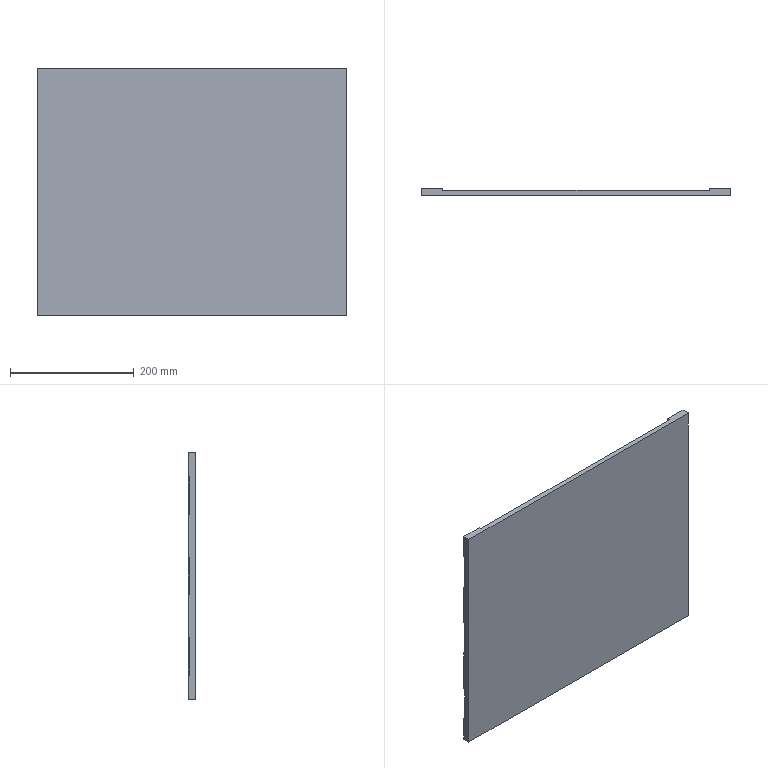Part | SolidWorks | features ICE 4, Extrusion 1, Fillet 1 | 1 solid | 28 faces | box 500 x 11.75 x 400 mm | volume 1696904 mm3 | plane 22 | cylinder 6 | commonest cylinder face diameters 10 x6
STEP:
#1=CARTESIAN_POINT('',(0.,9.75,-360.));
#2=VERTEX_POINT('',#1);
#3=CARTESIAN_POINT('',(0.,11.75,-360.));
#4=VERTEX_POINT('',#3);
#5=CARTESIAN_POINT('',(0.,9.75,-360.));
#6=DIRECTION('',(0.,1.,0.));
#7=VECTOR('',#6,1000.);
#8=LINE('',#5,#7);
#9=EDGE_CURVE('',#2,#4,#8,.T.);
#10=ORIENTED_EDGE('',*,*,#9,.T.);
#11=CARTESIAN_POINT('',(0.,11.75,-400.));
#12=VERTEX_POINT('',#11);
#13=CARTESIAN_POINT('',(0.,11.75,-400.));
#14=DIRECTION('',(0.,0.,1.));
#15=VECTOR('',#14,1000.);
#16=LINE('',#13,#15);
#17=EDGE_CURVE('',#12,#4,#16,.T.);
#18=ORIENTED_EDGE('',*,*,#17,.F.);
#19=CARTESIAN_POINT('',(0.,0.,-400.));
#20=VERTEX_POINT('',#19);
#21=CARTESIAN_POINT('',(0.,0.,-400.));
#22=DIRECTION('',(0.,-1.,0.));
#23=VECTOR('',#22,1000.);
#24=LINE('',#21,#23);
#25=EDGE_CURVE('',#12,#20,#24,.T.);
#26=ORIENTED_EDGE('',*,*,#25,.T.);
#27=CARTESIAN_POINT('',(0.,0.,0.));
#28=VERTEX_POINT('',#27);
#29=CARTESIAN_POINT('',(0.,0.,-400.));
#30=DIRECTION('',(0.,0.,1.));
#31=VECTOR('',#30,1000.);
#32=LINE('',#29,#31);
#33=EDGE_CURVE('',#20,#28,#32,.T.);
#34=ORIENTED_EDGE('',*,*,#33,.T.);
#35=CARTESIAN_POINT('',(0.,11.75,0.));
#36=VERTEX_POINT('',#35);
#37=CARTESIAN_POINT('',(0.,0.,0.));
#38=DIRECTION('',(0.,-1.,0.));
#39=VECTOR('',#38,1000.);
#40=LINE('',#37,#39);
#41=EDGE_CURVE('',#36,#28,#40,.T.);
#42=ORIENTED_EDGE('',*,*,#41,.F.);
#43=CARTESIAN_POINT('',(0.,11.75,-40.));
#44=VERTEX_POINT('',#43);
#45=CARTESIAN_POINT('',(0.,11.75,-400.));
#46=DIRECTION('',(0.,0.,1.));
#47=VECTOR('',#46,1000.);
#48=LINE('',#45,#47);
#49=EDGE_CURVE('',#44,#36,#48,.T.);
#50=ORIENTED_EDGE('',*,*,#49,.F.);
#51=CARTESIAN_POINT('',(0.,9.75,-40.));
#52=VERTEX_POINT('',#51);
#53=CARTESIAN_POINT('',(0.,9.75,-40.));
#54=DIRECTION('',(0.,1.,0.));
#55=VECTOR('',#54,1000.);
#56=LINE('',#53,#55);
#57=EDGE_CURVE('',#52,#44,#56,.T.);
#58=ORIENTED_EDGE('',*,*,#57,.F.);
#59=CARTESIAN_POINT('',(0.,9.75,-100.));
#60=VERTEX_POINT('',#59);
#61=CARTESIAN_POINT('',(0.,9.75,-40.));
#62=DIRECTION('',(0.,0.,1.));
#63=VECTOR('',#62,1000.);
#64=LINE('',#61,#63);
#65=EDGE_CURVE('',#60,#52,#64,.T.);
#66=ORIENTED_EDGE('',*,*,#65,.F.);
#67=CARTESIAN_POINT('',(0.,11.75,-100.));
#68=VERTEX_POINT('',#67);
#69=CARTESIAN_POINT('',(0.,9.75,-100.));
#70=DIRECTION('',(0.,1.,0.));
#71=VECTOR('',#70,1000.);
#72=LINE('',#69,#71);
#73=EDGE_CURVE('',#60,#68,#72,.T.);
#74=ORIENTED_EDGE('',*,*,#73,.T.);
#75=CARTESIAN_POINT('',(0.,11.75,-170.));
#76=VERTEX_POINT('',#75);
#77=CARTESIAN_POINT('',(0.,11.75,-400.));
#78=DIRECTION('',(0.,0.,1.));
#79=VECTOR('',#78,1000.);
#80=LINE('',#77,#79);
#81=EDGE_CURVE('',#76,#68,#80,.T.);
#82=ORIENTED_EDGE('',*,*,#81,.F.);
#83=CARTESIAN_POINT('',(0.,9.75,-170.));
#84=VERTEX_POINT('',#83);
#85=CARTESIAN_POINT('',(0.,9.75,-170.));
#86=DIRECTION('',(0.,1.,0.));
#87=VECTOR('',#86,1000.);
#88=LINE('',#85,#87);
#89=EDGE_CURVE('',#84,#76,#88,.T.);
#90=ORIENTED_EDGE('',*,*,#89,.F.);
#91=CARTESIAN_POINT('',(0.,9.75,-230.));
#92=VERTEX_POINT('',#91);
#93=CARTESIAN_POINT('',(0.,9.75,-230.));
#94=DIRECTION('',(0.,0.,1.));
#95=VECTOR('',#94,1000.);
#96=LINE('',#93,#95);
#97=EDGE_CURVE('',#92,#84,#96,.T.);
#98=ORIENTED_EDGE('',*,*,#97,.F.);
#99=CARTESIAN_POINT('',(0.,11.75,-230.));
#100=VERTEX_POINT('',#99);
#101=CARTESIAN_POINT('',(0.,9.75,-230.));
#102=DIRECTION('',(0.,1.,0.));
#103=VECTOR('',#102,1000.);
#104=LINE('',#101,#103);
#105=EDGE_CURVE('',#92,#100,#104,.T.);
#106=ORIENTED_EDGE('',*,*,#105,.T.);
#107=CARTESIAN_POINT('',(0.,11.75,-300.));
#108=VERTEX_POINT('',#107);
#109=CARTESIAN_POINT('',(0.,11.75,-400.));
#110=DIRECTION('',(0.,0.,1.));
#111=VECTOR('',#110,1000.);
#112=LINE('',#109,#111);
#113=EDGE_CURVE('',#108,#100,#112,.T.);
#114=ORIENTED_EDGE('',*,*,#113,.F.);
#115=CARTESIAN_POINT('',(0.,9.75,-300.));
#116=VERTEX_POINT('',#115);
#117=CARTESIAN_POINT('',(0.,9.75,-300.));
#118=DIRECTION('',(0.,1.,0.));
#119=VECTOR('',#118,1000.);
#120=LINE('',#117,#119);
#121=EDGE_CURVE('',#116,#108,#120,.T.);
#122=ORIENTED_EDGE('',*,*,#121,.F.);
#123=CARTESIAN_POINT('',(0.,9.75,-360.));
#124=DIRECTION('',(0.,0.,1.));
#125=VECTOR('',#124,1000.);
#126=LINE('',#123,#125);
#127=EDGE_CURVE('',#2,#116,#126,.T.);
#128=ORIENTED_EDGE('',*,*,#127,.F.);
#129=EDGE_LOOP('',(#10,#18,#26,#34,#42,#50,#58,#66,#74,#82,#90,#98,#106,#114,#122,#128));
#130=FACE_OUTER_BOUND('',#129,.T.);
#131=CARTESIAN_POINT('',(0.,0.,-400.));
#132=DIRECTION('',(-1.,0.,0.));
#133=DIRECTION('',(0.,0.,1.));
#134=AXIS2_PLACEMENT_3D('',#131,#132,#133);
#135=PLANE('',#134);
#136=ADVANCED_FACE('',(#130),#135,.T.);
#137=CARTESIAN_POINT('',(500.,11.75,0.));
#138=VERTEX_POINT('',#137);
#139=CARTESIAN_POINT('',(500.,11.75,-400.));
#140=VERTEX_POINT('',#139);
#141=CARTESIAN_POINT('',(500.,11.75,-400.));
#142=DIRECTION('',(0.,0.,-1.));
#143=VECTOR('',#142,1000.);
#144=LINE('',#141,#143);
#145=EDGE_CURVE('',#138,#140,#144,.T.);
#146=ORIENTED_EDGE('',*,*,#145,.F.);
#147=CARTESIAN_POINT('',(500.,0.,0.));
#148=VERTEX_POINT('',#147);
#149=CARTESIAN_POINT('',(500.,0.,0.));
#150=DIRECTION('',(0.,1.,0.));
#151=VECTOR('',#150,1000.);
#152=LINE('',#149,#151);
#153=EDGE_CURVE('',#148,#138,#152,.T.);
#154=ORIENTED_EDGE('',*,*,#153,.F.);
#155=CARTESIAN_POINT('',(500.,0.,-400.));
#156=VERTEX_POINT('',#155);
#157=CARTESIAN_POINT('',(500.,0.,-400.));
#158=DIRECTION('',(0.,0.,1.));
#159=VECTOR('',#158,1000.);
#160=LINE('',#157,#159);
#161=EDGE_CURVE('',#156,#148,#160,.T.);
#162=ORIENTED_EDGE('',*,*,#161,.F.);
#163=CARTESIAN_POINT('',(500.,0.,-400.));
#164=DIRECTION('',(0.,1.,0.));
#165=VECTOR('',#164,1000.);
#166=LINE('',#163,#165);
#167=EDGE_CURVE('',#156,#140,#166,.T.);
#168=ORIENTED_EDGE('',*,*,#167,.T.);
#169=EDGE_LOOP('',(#146,#154,#162,#168));
#170=FACE_OUTER_BOUND('',#169,.T.);
#171=CARTESIAN_POINT('',(500.,0.,-400.));
#172=DIRECTION('',(1.,0.,0.));
#173=DIRECTION('',(0.,0.,-1.));
#174=AXIS2_PLACEMENT_3D('',#171,#172,#173);
#175=PLANE('',#174);
#176=ADVANCED_FACE('',(#170),#175,.T.);
#177=CARTESIAN_POINT('',(465.,11.75,-400.));
#178=VERTEX_POINT('',#177);
#179=CARTESIAN_POINT('',(-22.479,11.75,-400.));
#180=DIRECTION('',(1.,0.,0.));
#181=VECTOR('',#180,1000.);
#182=LINE('',#179,#181);
#183=EDGE_CURVE('',#178,#140,#182,.T.);
#184=ORIENTED_EDGE('',*,*,#183,.T.);
#185=ORIENTED_EDGE('',*,*,#167,.F.);
#186=CARTESIAN_POINT('',(0.,0.,-400.));
#187=DIRECTION('',(1.,0.,0.));
#188=VECTOR('',#187,1000.);
#189=LINE('',#186,#188);
#190=EDGE_CURVE('',#20,#156,#189,.T.);
#191=ORIENTED_EDGE('',*,*,#190,.F.);
#192=ORIENTED_EDGE('',*,*,#25,.F.);
#193=CARTESIAN_POINT('',(35.,11.75,-400.));
#194=VERTEX_POINT('',#193);
#195=CARTESIAN_POINT('',(-22.479,11.75,-400.));
#196=DIRECTION('',(1.,0.,0.));
#197=VECTOR('',#196,1000.);
#198=LINE('',#195,#197);
#199=EDGE_CURVE('',#12,#194,#198,.T.);
#200=ORIENTED_EDGE('',*,*,#199,.T.);
#201=CARTESIAN_POINT('',(35.,8.,-400.));
#202=VERTEX_POINT('',#201);
#203=CARTESIAN_POINT('',(35.,16.,-400.));
#204=DIRECTION('',(0.,-1.,0.));
#205=VECTOR('',#204,1000.);
#206=LINE('',#203,#205);
#207=EDGE_CURVE('',#194,#202,#206,.T.);
#208=ORIENTED_EDGE('',*,*,#207,.T.);
#209=CARTESIAN_POINT('',(465.,8.,-400.));
#210=VERTEX_POINT('',#209);
#211=CARTESIAN_POINT('',(35.,8.,-400.));
#212=DIRECTION('',(1.,0.,0.));
#213=VECTOR('',#212,1000.);
#214=LINE('',#211,#213);
#215=EDGE_CURVE('',#202,#210,#214,.T.);
#216=ORIENTED_EDGE('',*,*,#215,.T.);
#217=CARTESIAN_POINT('',(465.,16.,-400.));
#218=DIRECTION('',(0.,1.,0.));
#219=VECTOR('',#218,1000.);
#220=LINE('',#217,#219);
#221=EDGE_CURVE('',#210,#178,#220,.T.);
#222=ORIENTED_EDGE('',*,*,#221,.T.);
#223=EDGE_LOOP('',(#184,#185,#191,#192,#200,#208,#216,#222));
#224=FACE_OUTER_BOUND('',#223,.T.);
#225=CARTESIAN_POINT('',(0.,0.,-400.));
#226=DIRECTION('',(0.,0.,-1.));
#227=DIRECTION('',(-1.,0.,0.));
#228=AXIS2_PLACEMENT_3D('',#225,#226,#227);
#229=PLANE('',#228);
#230=ADVANCED_FACE('',(#224),#229,.T.);
#231=ORIENTED_EDGE('',*,*,#153,.T.);
#232=CARTESIAN_POINT('',(465.,11.75,0.));
#233=VERTEX_POINT('',#232);
#234=CARTESIAN_POINT('',(-22.479,11.75,0.));
#235=DIRECTION('',(1.,0.,0.));
#236=VECTOR('',#235,1000.);
#237=LINE('',#234,#236);
#238=EDGE_CURVE('',#233,#138,#237,.T.);
#239=ORIENTED_EDGE('',*,*,#238,.F.);
#240=CARTESIAN_POINT('',(465.,8.,0.));
#241=VERTEX_POINT('',#240);
#242=CARTESIAN_POINT('',(465.,16.,0.));
#243=DIRECTION('',(0.,1.,0.));
#244=VECTOR('',#243,1000.);
#245=LINE('',#242,#244);
#246=EDGE_CURVE('',#241,#233,#245,.T.);
#247=ORIENTED_EDGE('',*,*,#246,.F.);
#248=CARTESIAN_POINT('',(35.,8.,0.));
#249=VERTEX_POINT('',#248);
#250=CARTESIAN_POINT('',(35.,8.,0.));
#251=DIRECTION('',(1.,0.,0.));
#252=VECTOR('',#251,1000.);
#253=LINE('',#250,#252);
#254=EDGE_CURVE('',#249,#241,#253,.T.);
#255=ORIENTED_EDGE('',*,*,#254,.F.);
#256=CARTESIAN_POINT('',(35.,11.75,0.));
#257=VERTEX_POINT('',#256);
#258=CARTESIAN_POINT('',(35.,16.,0.));
#259=DIRECTION('',(0.,-1.,0.));
#260=VECTOR('',#259,1000.);
#261=LINE('',#258,#260);
#262=EDGE_CURVE('',#257,#249,#261,.T.);
#263=ORIENTED_EDGE('',*,*,#262,.F.);
#264=CARTESIAN_POINT('',(-22.479,11.75,0.));
#265=DIRECTION('',(1.,0.,0.));
#266=VECTOR('',#265,1000.);
#267=LINE('',#264,#266);
#268=EDGE_CURVE('',#36,#257,#267,.T.);
#269=ORIENTED_EDGE('',*,*,#268,.F.);
#270=ORIENTED_EDGE('',*,*,#41,.T.);
#271=CARTESIAN_POINT('',(0.,0.,0.));
#272=DIRECTION('',(1.,0.,0.));
#273=VECTOR('',#272,1000.);
#274=LINE('',#271,#273);
#275=EDGE_CURVE('',#28,#148,#274,.T.);
#276=ORIENTED_EDGE('',*,*,#275,.T.);
#277=EDGE_LOOP('',(#231,#239,#247,#255,#263,#269,#270,#276));
#278=FACE_OUTER_BOUND('',#277,.T.);
#279=CARTESIAN_POINT('',(0.,0.,0.));
#280=DIRECTION('',(0.,0.,-1.));
#281=DIRECTION('',(-1.,0.,0.));
#282=AXIS2_PLACEMENT_3D('',#279,#280,#281);
#283=PLANE('',#282);
#284=ADVANCED_FACE('',(#278),#283,.F.);
#285=ORIENTED_EDGE('',*,*,#207,.F.);
#286=CARTESIAN_POINT('',(35.,11.75,-400.));
#287=DIRECTION('',(0.,0.,1.));
#288=VECTOR('',#287,1000.);
#289=LINE('',#286,#288);
#290=EDGE_CURVE('',#194,#257,#289,.T.);
#291=ORIENTED_EDGE('',*,*,#290,.T.);
#292=ORIENTED_EDGE('',*,*,#262,.T.);
#293=CARTESIAN_POINT('',(35.,8.,-400.));
#294=DIRECTION('',(0.,0.,1.));
#295=VECTOR('',#294,1000.);
#296=LINE('',#293,#295);
#297=EDGE_CURVE('',#202,#249,#296,.T.);
#298=ORIENTED_EDGE('',*,*,#297,.F.);
#299=EDGE_LOOP('',(#285,#291,#292,#298));
#300=FACE_OUTER_BOUND('',#299,.T.);
#301=CARTESIAN_POINT('',(35.,16.,-400.));
#302=DIRECTION('',(-1.,0.,0.));
#303=DIRECTION('',(0.,0.,1.));
#304=AXIS2_PLACEMENT_3D('',#301,#302,#303);
#305=PLANE('',#304);
#306=ADVANCED_FACE('',(#300),#305,.F.);
#307=ORIENTED_EDGE('',*,*,#246,.T.);
#308=CARTESIAN_POINT('',(465.,11.75,-400.));
#309=DIRECTION('',(0.,0.,-1.));
#310=VECTOR('',#309,1000.);
#311=LINE('',#308,#310);
#312=EDGE_CURVE('',#233,#178,#311,.T.);
#313=ORIENTED_EDGE('',*,*,#312,.T.);
#314=ORIENTED_EDGE('',*,*,#221,.F.);
#315=CARTESIAN_POINT('',(465.,8.,-400.));
#316=DIRECTION('',(0.,0.,1.));
#317=VECTOR('',#316,1000.);
#318=LINE('',#315,#317);
#319=EDGE_CURVE('',#210,#241,#318,.T.);
#320=ORIENTED_EDGE('',*,*,#319,.T.);
#321=EDGE_LOOP('',(#307,#313,#314,#320));
#322=FACE_OUTER_BOUND('',#321,.T.);
#323=CARTESIAN_POINT('',(465.,16.,-400.));
#324=DIRECTION('',(1.,0.,0.));
#325=DIRECTION('',(0.,0.,-1.));
#326=AXIS2_PLACEMENT_3D('',#323,#324,#325);
#327=PLANE('',#326);
#328=ADVANCED_FACE('',(#322),#327,.F.);
#329=ORIENTED_EDGE('',*,*,#275,.F.);
#330=ORIENTED_EDGE('',*,*,#33,.F.);
#331=ORIENTED_EDGE('',*,*,#190,.T.);
#332=ORIENTED_EDGE('',*,*,#161,.T.);
#333=EDGE_LOOP('',(#329,#330,#331,#332));
#334=FACE_OUTER_BOUND('',#333,.T.);
#335=CARTESIAN_POINT('',(0.,0.,-400.));
#336=DIRECTION('',(0.,-1.,0.));
#337=DIRECTION('',(0.,0.,-1.));
#338=AXIS2_PLACEMENT_3D('',#335,#336,#337);
#339=PLANE('',#338);
#340=ADVANCED_FACE('',(#334),#339,.T.);
#341=ORIENTED_EDGE('',*,*,#254,.T.);
#342=ORIENTED_EDGE('',*,*,#319,.F.);
#343=ORIENTED_EDGE('',*,*,#215,.F.);
#344=ORIENTED_EDGE('',*,*,#297,.T.);
#345=EDGE_LOOP('',(#341,#342,#343,#344));
#346=FACE_OUTER_BOUND('',#345,.T.);
#347=CARTESIAN_POINT('',(35.,8.,-400.));
#348=DIRECTION('',(0.,-1.,0.));
#349=DIRECTION('',(1.,0.,0.));
#350=AXIS2_PLACEMENT_3D('',#347,#348,#349);
#351=PLANE('',#350);
#352=ADVANCED_FACE('',(#346),#351,.F.);
#353=ORIENTED_EDGE('',*,*,#145,.T.);
#354=ORIENTED_EDGE('',*,*,#183,.F.);
#355=ORIENTED_EDGE('',*,*,#312,.F.);
#356=ORIENTED_EDGE('',*,*,#238,.T.);
#357=EDGE_LOOP('',(#353,#354,#355,#356));
#358=FACE_OUTER_BOUND('',#357,.T.);
#359=CARTESIAN_POINT('',(-22.479,11.75,-400.));
#360=DIRECTION('',(0.,-1.,0.));
#361=DIRECTION('',(0.,0.,-1.));
#362=AXIS2_PLACEMENT_3D('',#359,#360,#361);
#363=PLANE('',#362);
#364=ADVANCED_FACE('',(#358),#363,.F.);
#365=ORIENTED_EDGE('',*,*,#17,.T.);
#366=CARTESIAN_POINT('',(19.,11.75,-360.));
#367=VERTEX_POINT('',#366);
#368=CARTESIAN_POINT('',(0.,11.75,-360.));
#369=DIRECTION('',(-1.,0.,0.));
#370=VECTOR('',#369,1000.);
#371=LINE('',#368,#370);
#372=EDGE_CURVE('',#367,#4,#371,.T.);
#373=ORIENTED_EDGE('',*,*,#372,.F.);
#374=CARTESIAN_POINT('',(24.,11.75,-355.));
#375=VERTEX_POINT('',#374);
#376=CARTESIAN_POINT('',(19.,11.75,-355.));
#377=DIRECTION('',(0.,-1.,0.));
#378=DIRECTION('',(0.,0.,-1.));
#379=AXIS2_PLACEMENT_3D('',#376,#377,#378);
#380=CIRCLE('',#379,5.);
#381=EDGE_CURVE('',#367,#375,#380,.T.);
#382=ORIENTED_EDGE('',*,*,#381,.T.);
#383=CARTESIAN_POINT('',(24.,11.75,-305.));
#384=VERTEX_POINT('',#383);
#385=CARTESIAN_POINT('',(24.,11.75,-360.));
#386=DIRECTION('',(0.,0.,-1.));
#387=VECTOR('',#386,1000.);
#388=LINE('',#385,#387);
#389=EDGE_CURVE('',#384,#375,#388,.T.);
#390=ORIENTED_EDGE('',*,*,#389,.F.);
#391=CARTESIAN_POINT('',(19.,11.75,-300.));
#392=VERTEX_POINT('',#391);
#393=CARTESIAN_POINT('',(19.,11.75,-305.));
#394=DIRECTION('',(0.,-1.,0.));
#395=DIRECTION('',(0.,0.,-1.));
#396=AXIS2_PLACEMENT_3D('',#393,#394,#395);
#397=CIRCLE('',#396,5.);
#398=EDGE_CURVE('',#384,#392,#397,.T.);
#399=ORIENTED_EDGE('',*,*,#398,.T.);
#400=CARTESIAN_POINT('',(0.,11.75,-300.));
#401=DIRECTION('',(1.,0.,0.));
#402=VECTOR('',#401,1000.);
#403=LINE('',#400,#402);
#404=EDGE_CURVE('',#108,#392,#403,.T.);
#405=ORIENTED_EDGE('',*,*,#404,.F.);
#406=ORIENTED_EDGE('',*,*,#113,.T.);
#407=CARTESIAN_POINT('',(15.,11.75,-230.));
#408=VERTEX_POINT('',#407);
#409=CARTESIAN_POINT('',(20.,11.75,-230.));
#410=DIRECTION('',(-1.,0.,0.));
#411=VECTOR('',#410,1000.);
#412=LINE('',#409,#411);
#413=EDGE_CURVE('',#408,#100,#412,.T.);
#414=ORIENTED_EDGE('',*,*,#413,.F.);
#415=CARTESIAN_POINT('',(20.,11.75,-225.));
#416=VERTEX_POINT('',#415);
#417=CARTESIAN_POINT('',(15.,11.75,-225.));
#418=DIRECTION('',(0.,-1.,0.));
#419=DIRECTION('',(0.,0.,-1.));
#420=AXIS2_PLACEMENT_3D('',#417,#418,#419);
#421=CIRCLE('',#420,5.);
#422=EDGE_CURVE('',#408,#416,#421,.T.);
#423=ORIENTED_EDGE('',*,*,#422,.T.);
#424=CARTESIAN_POINT('',(20.,11.75,-175.));
#425=VERTEX_POINT('',#424);
#426=CARTESIAN_POINT('',(20.,11.75,-230.));
#427=DIRECTION('',(0.,0.,-1.));
#428=VECTOR('',#427,1000.);
#429=LINE('',#426,#428);
#430=EDGE_CURVE('',#425,#416,#429,.T.);
#431=ORIENTED_EDGE('',*,*,#430,.F.);
#432=CARTESIAN_POINT('',(15.,11.75,-170.));
#433=VERTEX_POINT('',#432);
#434=CARTESIAN_POINT('',(15.,11.75,-175.));
#435=DIRECTION('',(0.,-1.,0.));
#436=DIRECTION('',(0.,0.,-1.));
#437=AXIS2_PLACEMENT_3D('',#434,#435,#436);
#438=CIRCLE('',#437,5.);
#439=EDGE_CURVE('',#425,#433,#438,.T.);
#440=ORIENTED_EDGE('',*,*,#439,.T.);
#441=CARTESIAN_POINT('',(20.,11.75,-170.));
#442=DIRECTION('',(1.,0.,0.));
#443=VECTOR('',#442,1000.);
#444=LINE('',#441,#443);
#445=EDGE_CURVE('',#76,#433,#444,.T.);
#446=ORIENTED_EDGE('',*,*,#445,.F.);
#447=ORIENTED_EDGE('',*,*,#81,.T.);
#448=CARTESIAN_POINT('',(19.,11.75,-100.));
#449=VERTEX_POINT('',#448);
#450=CARTESIAN_POINT('',(0.,11.75,-100.));
#451=DIRECTION('',(-1.,0.,0.));
#452=VECTOR('',#451,1000.);
#453=LINE('',#450,#452);
#454=EDGE_CURVE('',#449,#68,#453,.T.);
#455=ORIENTED_EDGE('',*,*,#454,.F.);
#456=CARTESIAN_POINT('',(24.,11.75,-95.));
#457=VERTEX_POINT('',#456);
#458=CARTESIAN_POINT('',(19.,11.75,-95.));
#459=DIRECTION('',(0.,-1.,0.));
#460=DIRECTION('',(0.,0.,-1.));
#461=AXIS2_PLACEMENT_3D('',#458,#459,#460);
#462=CIRCLE('',#461,5.);
#463=EDGE_CURVE('',#449,#457,#462,.T.);
#464=ORIENTED_EDGE('',*,*,#463,.T.);
#465=CARTESIAN_POINT('',(24.,11.75,-45.));
#466=VERTEX_POINT('',#465);
#467=CARTESIAN_POINT('',(24.,11.75,-40.));
#468=DIRECTION('',(0.,0.,-1.));
#469=VECTOR('',#468,1000.);
#470=LINE('',#467,#469);
#471=EDGE_CURVE('',#466,#457,#470,.T.);
#472=ORIENTED_EDGE('',*,*,#471,.F.);
#473=CARTESIAN_POINT('',(19.,11.75,-40.));
#474=VERTEX_POINT('',#473);
#475=CARTESIAN_POINT('',(19.,11.75,-45.));
#476=DIRECTION('',(0.,-1.,0.));
#477=DIRECTION('',(0.,0.,-1.));
#478=AXIS2_PLACEMENT_3D('',#475,#476,#477);
#479=CIRCLE('',#478,5.);
#480=EDGE_CURVE('',#466,#474,#479,.T.);
#481=ORIENTED_EDGE('',*,*,#480,.T.);
#482=CARTESIAN_POINT('',(0.,11.75,-40.));
#483=DIRECTION('',(1.,0.,0.));
#484=VECTOR('',#483,1000.);
#485=LINE('',#482,#484);
#486=EDGE_CURVE('',#44,#474,#485,.T.);
#487=ORIENTED_EDGE('',*,*,#486,.F.);
#488=ORIENTED_EDGE('',*,*,#49,.T.);
#489=ORIENTED_EDGE('',*,*,#268,.T.);
#490=ORIENTED_EDGE('',*,*,#290,.F.);
#491=ORIENTED_EDGE('',*,*,#199,.F.);
#492=EDGE_LOOP('',(#365,#373,#382,#390,#399,#405,#406,#414,#423,#431,#440,#446,#447,#455,#464,#472,#481,#487,#488,#489,#490,#491));
#493=FACE_OUTER_BOUND('',#492,.T.);
#494=CARTESIAN_POINT('',(-22.479,11.75,-400.));
#495=DIRECTION('',(0.,-1.,0.));
#496=DIRECTION('',(0.,0.,-1.));
#497=AXIS2_PLACEMENT_3D('',#494,#495,#496);
#498=PLANE('',#497);
#499=ADVANCED_FACE('',(#493),#498,.F.);
#500=CARTESIAN_POINT('',(20.,9.75,-175.));
#501=VERTEX_POINT('',#500);
#502=CARTESIAN_POINT('',(20.,9.75,-225.));
#503=VERTEX_POINT('',#502);
#504=CARTESIAN_POINT('',(20.,9.75,-230.));
#505=DIRECTION('',(0.,0.,-1.));
#506=VECTOR('',#505,1000.);
#507=LINE('',#504,#506);
#508=EDGE_CURVE('',#501,#503,#507,.T.);
#509=ORIENTED_EDGE('',*,*,#508,.F.);
#510=CARTESIAN_POINT('',(20.,11.75,-175.));
#511=DIRECTION('',(0.,1.,0.));
#512=VECTOR('',#511,1000.);
#513=LINE('',#510,#512);
#514=EDGE_CURVE('',#501,#425,#513,.T.);
#515=ORIENTED_EDGE('',*,*,#514,.T.);
#516=ORIENTED_EDGE('',*,*,#430,.T.);
#517=CARTESIAN_POINT('',(20.,9.75,-225.));
#518=DIRECTION('',(0.,-1.,0.));
#519=VECTOR('',#518,1000.);
#520=LINE('',#517,#519);
#521=EDGE_CURVE('',#416,#503,#520,.T.);
#522=ORIENTED_EDGE('',*,*,#521,.T.);
#523=EDGE_LOOP('',(#509,#515,#516,#522));
#524=FACE_OUTER_BOUND('',#523,.T.);
#525=CARTESIAN_POINT('',(20.,9.75,-230.));
#526=DIRECTION('',(1.,0.,0.));
#527=DIRECTION('',(0.,0.,-1.));
#528=AXIS2_PLACEMENT_3D('',#525,#526,#527);
#529=PLANE('',#528);
#530=ADVANCED_FACE('',(#524),#529,.F.);
#531=ORIENTED_EDGE('',*,*,#445,.T.);
#532=CARTESIAN_POINT('',(15.,9.75,-170.));
#533=VERTEX_POINT('',#532);
#534=CARTESIAN_POINT('',(15.,9.75,-170.));
#535=DIRECTION('',(0.,-1.,0.));
#536=VECTOR('',#535,1000.);
#537=LINE('',#534,#536);
#538=EDGE_CURVE('',#433,#533,#537,.T.);
#539=ORIENTED_EDGE('',*,*,#538,.T.);
#540=CARTESIAN_POINT('',(20.,9.75,-170.));
#541=DIRECTION('',(1.,0.,0.));
#542=VECTOR('',#541,1000.);
#543=LINE('',#540,#542);
#544=EDGE_CURVE('',#84,#533,#543,.T.);
#545=ORIENTED_EDGE('',*,*,#544,.F.);
#546=ORIENTED_EDGE('',*,*,#89,.T.);
#547=EDGE_LOOP('',(#531,#539,#545,#546));
#548=FACE_OUTER_BOUND('',#547,.T.);
#549=CARTESIAN_POINT('',(20.,9.75,-170.));
#550=DIRECTION('',(0.,0.,1.));
#551=DIRECTION('',(1.,0.,0.));
#552=AXIS2_PLACEMENT_3D('',#549,#550,#551);
#553=PLANE('',#552);
#554=ADVANCED_FACE('',(#548),#553,.F.);
#555=CARTESIAN_POINT('',(15.,9.75,-230.));
#556=VERTEX_POINT('',#555);
#557=CARTESIAN_POINT('',(20.,9.75,-230.));
#558=DIRECTION('',(-1.,0.,0.));
#559=VECTOR('',#558,1000.);
#560=LINE('',#557,#559);
#561=EDGE_CURVE('',#556,#92,#560,.T.);
#562=ORIENTED_EDGE('',*,*,#561,.F.);
#563=CARTESIAN_POINT('',(15.,11.75,-230.));
#564=DIRECTION('',(0.,1.,0.));
#565=VECTOR('',#564,1000.);
#566=LINE('',#563,#565);
#567=EDGE_CURVE('',#556,#408,#566,.T.);
#568=ORIENTED_EDGE('',*,*,#567,.T.);
#569=ORIENTED_EDGE('',*,*,#413,.T.);
#570=ORIENTED_EDGE('',*,*,#105,.F.);
#571=EDGE_LOOP('',(#562,#568,#569,#570));
#572=FACE_OUTER_BOUND('',#571,.T.);
#573=CARTESIAN_POINT('',(20.,9.75,-230.));
#574=DIRECTION('',(0.,0.,-1.));
#575=DIRECTION('',(-1.,0.,0.));
#576=AXIS2_PLACEMENT_3D('',#573,#574,#575);
#577=PLANE('',#576);
#578=ADVANCED_FACE('',(#572),#577,.F.);
#579=ORIENTED_EDGE('',*,*,#544,.T.);
#580=CARTESIAN_POINT('',(15.,9.75,-175.));
#581=DIRECTION('',(0.,1.,0.));
#582=DIRECTION('',(0.,0.,-1.));
#583=AXIS2_PLACEMENT_3D('',#580,#581,#582);
#584=CIRCLE('',#583,5.);
#585=EDGE_CURVE('',#533,#501,#584,.T.);
#586=ORIENTED_EDGE('',*,*,#585,.T.);
#587=ORIENTED_EDGE('',*,*,#508,.T.);
#588=CARTESIAN_POINT('',(15.,9.75,-225.));
#589=DIRECTION('',(0.,1.,0.));
#590=DIRECTION('',(0.,0.,-1.));
#591=AXIS2_PLACEMENT_3D('',#588,#589,#590);
#592=CIRCLE('',#591,5.);
#593=EDGE_CURVE('',#503,#556,#592,.T.);
#594=ORIENTED_EDGE('',*,*,#593,.T.);
#595=ORIENTED_EDGE('',*,*,#561,.T.);
#596=ORIENTED_EDGE('',*,*,#97,.T.);
#597=EDGE_LOOP('',(#579,#586,#587,#594,#595,#596));
#598=FACE_OUTER_BOUND('',#597,.T.);
#599=CARTESIAN_POINT('',(0.,9.75,0.));
#600=DIRECTION('',(0.,-1.,0.));
#601=DIRECTION('',(0.,0.,-1.));
#602=AXIS2_PLACEMENT_3D('',#599,#600,#601);
#603=PLANE('',#602);
#604=ADVANCED_FACE('',(#598),#603,.F.);
#605=ORIENTED_EDGE('',*,*,#486,.T.);
#606=CARTESIAN_POINT('',(19.,9.75,-40.));
#607=VERTEX_POINT('',#606);
#608=CARTESIAN_POINT('',(19.,9.75,-40.));
#609=DIRECTION('',(0.,-1.,0.));
#610=VECTOR('',#609,1000.);
#611=LINE('',#608,#610);
#612=EDGE_CURVE('',#474,#607,#611,.T.);
#613=ORIENTED_EDGE('',*,*,#612,.T.);
#614=CARTESIAN_POINT('',(0.,9.75,-40.));
#615=DIRECTION('',(1.,0.,0.));
#616=VECTOR('',#615,1000.);
#617=LINE('',#614,#616);
#618=EDGE_CURVE('',#52,#607,#617,.T.);
#619=ORIENTED_EDGE('',*,*,#618,.F.);
#620=ORIENTED_EDGE('',*,*,#57,.T.);
#621=EDGE_LOOP('',(#605,#613,#619,#620));
#622=FACE_OUTER_BOUND('',#621,.T.);
#623=CARTESIAN_POINT('',(0.,9.75,-40.));
#624=DIRECTION('',(0.,0.,1.));
#625=DIRECTION('',(1.,0.,0.));
#626=AXIS2_PLACEMENT_3D('',#623,#624,#625);
#627=PLANE('',#626);
#628=ADVANCED_FACE('',(#622),#627,.F.);
#629=CARTESIAN_POINT('',(19.,9.75,-100.));
#630=VERTEX_POINT('',#629);
#631=CARTESIAN_POINT('',(0.,9.75,-100.));
#632=DIRECTION('',(-1.,0.,0.));
#633=VECTOR('',#632,1000.);
#634=LINE('',#631,#633);
#635=EDGE_CURVE('',#630,#60,#634,.T.);
#636=ORIENTED_EDGE('',*,*,#635,.F.);
#637=CARTESIAN_POINT('',(19.,11.75,-100.));
#638=DIRECTION('',(0.,1.,0.));
#639=VECTOR('',#638,1000.);
#640=LINE('',#637,#639);
#641=EDGE_CURVE('',#630,#449,#640,.T.);
#642=ORIENTED_EDGE('',*,*,#641,.T.);
#643=ORIENTED_EDGE('',*,*,#454,.T.);
#644=ORIENTED_EDGE('',*,*,#73,.F.);
#645=EDGE_LOOP('',(#636,#642,#643,#644));
#646=FACE_OUTER_BOUND('',#645,.T.);
#647=CARTESIAN_POINT('',(0.,9.75,-100.));
#648=DIRECTION('',(0.,0.,-1.));
#649=DIRECTION('',(-1.,0.,0.));
#650=AXIS2_PLACEMENT_3D('',#647,#648,#649);
#651=PLANE('',#650);
#652=ADVANCED_FACE('',(#646),#651,.F.);
#653=CARTESIAN_POINT('',(24.,9.75,-45.));
#654=VERTEX_POINT('',#653);
#655=CARTESIAN_POINT('',(24.,9.75,-95.));
#656=VERTEX_POINT('',#655);
#657=CARTESIAN_POINT('',(24.,9.75,-40.));
#658=DIRECTION('',(0.,0.,-1.));
#659=VECTOR('',#658,1000.);
#660=LINE('',#657,#659);
#661=EDGE_CURVE('',#654,#656,#660,.T.);
#662=ORIENTED_EDGE('',*,*,#661,.F.);
#663=CARTESIAN_POINT('',(24.,11.75,-45.));
#664=DIRECTION('',(0.,1.,0.));
#665=VECTOR('',#664,1000.);
#666=LINE('',#663,#665);
#667=EDGE_CURVE('',#654,#466,#666,.T.);
#668=ORIENTED_EDGE('',*,*,#667,.T.);
#669=ORIENTED_EDGE('',*,*,#471,.T.);
#670=CARTESIAN_POINT('',(24.,9.75,-95.));
#671=DIRECTION('',(0.,-1.,0.));
#672=VECTOR('',#671,1000.);
#673=LINE('',#670,#672);
#674=EDGE_CURVE('',#457,#656,#673,.T.);
#675=ORIENTED_EDGE('',*,*,#674,.T.);
#676=EDGE_LOOP('',(#662,#668,#669,#675));
#677=FACE_OUTER_BOUND('',#676,.T.);
#678=CARTESIAN_POINT('',(24.,9.75,-40.));
#679=DIRECTION('',(1.,0.,0.));
#680=DIRECTION('',(0.,0.,-1.));
#681=AXIS2_PLACEMENT_3D('',#678,#679,#680);
#682=PLANE('',#681);
#683=ADVANCED_FACE('',(#677),#682,.F.);
#684=ORIENTED_EDGE('',*,*,#618,.T.);
#685=CARTESIAN_POINT('',(19.,9.75,-45.));
#686=DIRECTION('',(0.,1.,0.));
#687=DIRECTION('',(0.,0.,1.));
#688=AXIS2_PLACEMENT_3D('',#685,#686,#687);
#689=CIRCLE('',#688,5.);
#690=EDGE_CURVE('',#607,#654,#689,.T.);
#691=ORIENTED_EDGE('',*,*,#690,.T.);
#692=ORIENTED_EDGE('',*,*,#661,.T.);
#693=CARTESIAN_POINT('',(19.,9.75,-95.));
#694=DIRECTION('',(0.,1.,0.));
#695=DIRECTION('',(0.,0.,1.));
#696=AXIS2_PLACEMENT_3D('',#693,#694,#695);
#697=CIRCLE('',#696,5.);
#698=EDGE_CURVE('',#656,#630,#697,.T.);
#699=ORIENTED_EDGE('',*,*,#698,.T.);
#700=ORIENTED_EDGE('',*,*,#635,.T.);
#701=ORIENTED_EDGE('',*,*,#65,.T.);
#702=EDGE_LOOP('',(#684,#691,#692,#699,#700,#701));
#703=FACE_OUTER_BOUND('',#702,.T.);
#704=CARTESIAN_POINT('',(0.,9.75,0.));
#705=DIRECTION('',(0.,1.,0.));
#706=DIRECTION('',(0.,0.,1.));
#707=AXIS2_PLACEMENT_3D('',#704,#705,#706);
#708=PLANE('',#707);
#709=ADVANCED_FACE('',(#703),#708,.T.);
#710=CARTESIAN_POINT('',(19.,9.75,-360.));
#711=VERTEX_POINT('',#710);
#712=CARTESIAN_POINT('',(0.,9.75,-360.));
#713=DIRECTION('',(-1.,0.,0.));
#714=VECTOR('',#713,1000.);
#715=LINE('',#712,#714);
#716=EDGE_CURVE('',#711,#2,#715,.T.);
#717=ORIENTED_EDGE('',*,*,#716,.F.);
#718=CARTESIAN_POINT('',(19.,11.75,-360.));
#719=DIRECTION('',(0.,1.,0.));
#720=VECTOR('',#719,1000.);
#721=LINE('',#718,#720);
#722=EDGE_CURVE('',#711,#367,#721,.T.);
#723=ORIENTED_EDGE('',*,*,#722,.T.);
#724=ORIENTED_EDGE('',*,*,#372,.T.);
#725=ORIENTED_EDGE('',*,*,#9,.F.);
#726=EDGE_LOOP('',(#717,#723,#724,#725));
#727=FACE_OUTER_BOUND('',#726,.T.);
#728=CARTESIAN_POINT('',(0.,9.75,-360.));
#729=DIRECTION('',(0.,0.,-1.));
#730=DIRECTION('',(-1.,0.,0.));
#731=AXIS2_PLACEMENT_3D('',#728,#729,#730);
#732=PLANE('',#731);
#733=ADVANCED_FACE('',(#727),#732,.F.);
#734=CARTESIAN_POINT('',(24.,9.75,-305.));
#735=VERTEX_POINT('',#734);
#736=CARTESIAN_POINT('',(24.,9.75,-355.));
#737=VERTEX_POINT('',#736);
#738=CARTESIAN_POINT('',(24.,9.75,-360.));
#739=DIRECTION('',(0.,0.,-1.));
#740=VECTOR('',#739,1000.);
#741=LINE('',#738,#740);
#742=EDGE_CURVE('',#735,#737,#741,.T.);
#743=ORIENTED_EDGE('',*,*,#742,.F.);
#744=CARTESIAN_POINT('',(24.,11.75,-305.));
#745=DIRECTION('',(0.,1.,0.));
#746=VECTOR('',#745,1000.);
#747=LINE('',#744,#746);
#748=EDGE_CURVE('',#735,#384,#747,.T.);
#749=ORIENTED_EDGE('',*,*,#748,.T.);
#750=ORIENTED_EDGE('',*,*,#389,.T.);
#751=CARTESIAN_POINT('',(24.,9.75,-355.));
#752=DIRECTION('',(0.,-1.,0.));
#753=VECTOR('',#752,1000.);
#754=LINE('',#751,#753);
#755=EDGE_CURVE('',#375,#737,#754,.T.);
#756=ORIENTED_EDGE('',*,*,#755,.T.);
#757=EDGE_LOOP('',(#743,#749,#750,#756));
#758=FACE_OUTER_BOUND('',#757,.T.);
#759=CARTESIAN_POINT('',(24.,9.75,-360.));
#760=DIRECTION('',(1.,0.,0.));
#761=DIRECTION('',(0.,0.,-1.));
#762=AXIS2_PLACEMENT_3D('',#759,#760,#761);
#763=PLANE('',#762);
#764=ADVANCED_FACE('',(#758),#763,.F.);
#765=ORIENTED_EDGE('',*,*,#404,.T.);
#766=CARTESIAN_POINT('',(19.,9.75,-300.));
#767=VERTEX_POINT('',#766);
#768=CARTESIAN_POINT('',(19.,9.75,-300.));
#769=DIRECTION('',(0.,-1.,0.));
#770=VECTOR('',#769,1000.);
#771=LINE('',#768,#770);
#772=EDGE_CURVE('',#392,#767,#771,.T.);
#773=ORIENTED_EDGE('',*,*,#772,.T.);
#774=CARTESIAN_POINT('',(0.,9.75,-300.));
#775=DIRECTION('',(1.,0.,0.));
#776=VECTOR('',#775,1000.);
#777=LINE('',#774,#776);
#778=EDGE_CURVE('',#116,#767,#777,.T.);
#779=ORIENTED_EDGE('',*,*,#778,.F.);
#780=ORIENTED_EDGE('',*,*,#121,.T.);
#781=EDGE_LOOP('',(#765,#773,#779,#780));
#782=FACE_OUTER_BOUND('',#781,.T.);
#783=CARTESIAN_POINT('',(0.,9.75,-300.));
#784=DIRECTION('',(0.,0.,1.));
#785=DIRECTION('',(1.,0.,0.));
#786=AXIS2_PLACEMENT_3D('',#783,#784,#785);
#787=PLANE('',#786);
#788=ADVANCED_FACE('',(#782),#787,.F.);
#789=ORIENTED_EDGE('',*,*,#778,.T.);
#790=CARTESIAN_POINT('',(19.,9.75,-305.));
#791=DIRECTION('',(0.,1.,0.));
#792=DIRECTION('',(0.,0.,1.));
#793=AXIS2_PLACEMENT_3D('',#790,#791,#792);
#794=CIRCLE('',#793,5.);
#795=EDGE_CURVE('',#767,#735,#794,.T.);
#796=ORIENTED_EDGE('',*,*,#795,.T.);
#797=ORIENTED_EDGE('',*,*,#742,.T.);
#798=CARTESIAN_POINT('',(19.,9.75,-355.));
#799=DIRECTION('',(0.,1.,0.));
#800=DIRECTION('',(0.,0.,1.));
#801=AXIS2_PLACEMENT_3D('',#798,#799,#800);
#802=CIRCLE('',#801,5.);
#803=EDGE_CURVE('',#737,#711,#802,.T.);
#804=ORIENTED_EDGE('',*,*,#803,.T.);
#805=ORIENTED_EDGE('',*,*,#716,.T.);
#806=ORIENTED_EDGE('',*,*,#127,.T.);
#807=EDGE_LOOP('',(#789,#796,#797,#804,#805,#806));
#808=FACE_OUTER_BOUND('',#807,.T.);
#809=CARTESIAN_POINT('',(0.,9.75,0.));
#810=DIRECTION('',(0.,1.,0.));
#811=DIRECTION('',(0.,0.,1.));
#812=AXIS2_PLACEMENT_3D('',#809,#810,#811);
#813=PLANE('',#812);
#814=ADVANCED_FACE('',(#808),#813,.T.);
#815=ORIENTED_EDGE('',*,*,#690,.F.);
#816=ORIENTED_EDGE('',*,*,#612,.F.);
#817=ORIENTED_EDGE('',*,*,#480,.F.);
#818=ORIENTED_EDGE('',*,*,#667,.F.);
#819=EDGE_LOOP('',(#815,#816,#817,#818));
#820=FACE_OUTER_BOUND('',#819,.T.);
#821=CARTESIAN_POINT('',(19.,9.75,-45.));
#822=DIRECTION('',(0.,-1.,0.));
#823=DIRECTION('',(0.,0.,-1.));
#824=AXIS2_PLACEMENT_3D('',#821,#822,#823);
#825=CYLINDRICAL_SURFACE('',#824,5.);
#826=ADVANCED_FACE('',(#820),#825,.F.);
#827=ORIENTED_EDGE('',*,*,#698,.F.);
#828=ORIENTED_EDGE('',*,*,#674,.F.);
#829=ORIENTED_EDGE('',*,*,#463,.F.);
#830=ORIENTED_EDGE('',*,*,#641,.F.);
#831=EDGE_LOOP('',(#827,#828,#829,#830));
#832=FACE_OUTER_BOUND('',#831,.T.);
#833=CARTESIAN_POINT('',(19.,9.75,-95.));
#834=DIRECTION('',(0.,-1.,0.));
#835=DIRECTION('',(0.,0.,-1.));
#836=AXIS2_PLACEMENT_3D('',#833,#834,#835);
#837=CYLINDRICAL_SURFACE('',#836,5.);
#838=ADVANCED_FACE('',(#832),#837,.F.);
#839=ORIENTED_EDGE('',*,*,#585,.F.);
#840=ORIENTED_EDGE('',*,*,#538,.F.);
#841=ORIENTED_EDGE('',*,*,#439,.F.);
#842=ORIENTED_EDGE('',*,*,#514,.F.);
#843=EDGE_LOOP('',(#839,#840,#841,#842));
#844=FACE_OUTER_BOUND('',#843,.T.);
#845=CARTESIAN_POINT('',(15.,9.75,-175.));
#846=DIRECTION('',(0.,-1.,0.));
#847=DIRECTION('',(0.,0.,-1.));
#848=AXIS2_PLACEMENT_3D('',#845,#846,#847);
#849=CYLINDRICAL_SURFACE('',#848,5.);
#850=ADVANCED_FACE('',(#844),#849,.F.);
#851=ORIENTED_EDGE('',*,*,#593,.F.);
#852=ORIENTED_EDGE('',*,*,#521,.F.);
#853=ORIENTED_EDGE('',*,*,#422,.F.);
#854=ORIENTED_EDGE('',*,*,#567,.F.);
#855=EDGE_LOOP('',(#851,#852,#853,#854));
#856=FACE_OUTER_BOUND('',#855,.T.);
#857=CARTESIAN_POINT('',(15.,9.75,-225.));
#858=DIRECTION('',(0.,-1.,0.));
#859=DIRECTION('',(0.,0.,-1.));
#860=AXIS2_PLACEMENT_3D('',#857,#858,#859);
#861=CYLINDRICAL_SURFACE('',#860,5.);
#862=ADVANCED_FACE('',(#856),#861,.F.);
#863=ORIENTED_EDGE('',*,*,#795,.F.);
#864=ORIENTED_EDGE('',*,*,#772,.F.);
#865=ORIENTED_EDGE('',*,*,#398,.F.);
#866=ORIENTED_EDGE('',*,*,#748,.F.);
#867=EDGE_LOOP('',(#863,#864,#865,#866));
#868=FACE_OUTER_BOUND('',#867,.T.);
#869=CARTESIAN_POINT('',(19.,9.75,-305.));
#870=DIRECTION('',(0.,-1.,0.));
#871=DIRECTION('',(0.,0.,-1.));
#872=AXIS2_PLACEMENT_3D('',#869,#870,#871);
#873=CYLINDRICAL_SURFACE('',#872,5.);
#874=ADVANCED_FACE('',(#868),#873,.F.);
#875=ORIENTED_EDGE('',*,*,#803,.F.);
#876=ORIENTED_EDGE('',*,*,#755,.F.);
#877=ORIENTED_EDGE('',*,*,#381,.F.);
#878=ORIENTED_EDGE('',*,*,#722,.F.);
#879=EDGE_LOOP('',(#875,#876,#877,#878));
#880=FACE_OUTER_BOUND('',#879,.T.);
#881=CARTESIAN_POINT('',(19.,9.75,-355.));
#882=DIRECTION('',(0.,-1.,0.));
#883=DIRECTION('',(0.,0.,-1.));
#884=AXIS2_PLACEMENT_3D('',#881,#882,#883);
#885=CYLINDRICAL_SURFACE('',#884,5.);
#886=ADVANCED_FACE('',(#880),#885,.F.);
#887=CLOSED_SHELL('',(#136,#176,#230,#284,#306,#328,#340,#352,#364,#499,#530,#554,#578,#604,#628,#652,#683,#709,#733,#764,#788,#814,#826,#838,#850,#862,#874,#886));
#888=MANIFOLD_SOLID_BREP('',#887);
#889=CARTESIAN_POINT('',(0.,0.,0.));
#890=DIRECTION('',(0.,0.,1.));
#891=DIRECTION('',(1.,0.,0.));
#892=AXIS2_PLACEMENT_3D('',#889,#890,#891);
#893=(LENGTH_UNIT()NAMED_UNIT(*)SI_UNIT(.MILLI.,.METRE.));
#894=UNCERTAINTY_MEASURE_WITH_UNIT(LENGTH_MEASURE(0.00001),#893,'','');
#895=(NAMED_UNIT(*)PLANE_ANGLE_UNIT()SI_UNIT($,.RADIAN.));
#896=(NAMED_UNIT(*)SI_UNIT($,.STERADIAN.)SOLID_ANGLE_UNIT());
#897=(GEOMETRIC_REPRESENTATION_CONTEXT(3)GLOBAL_UNCERTAINTY_ASSIGNED_CONTEXT((#894))GLOBAL_UNIT_ASSIGNED_CONTEXT((#893,#895,#896))REPRESENTATION_CONTEXT('',''));
#898=ADVANCED_BREP_SHAPE_REPRESENTATION('',(#888,#892),#897);